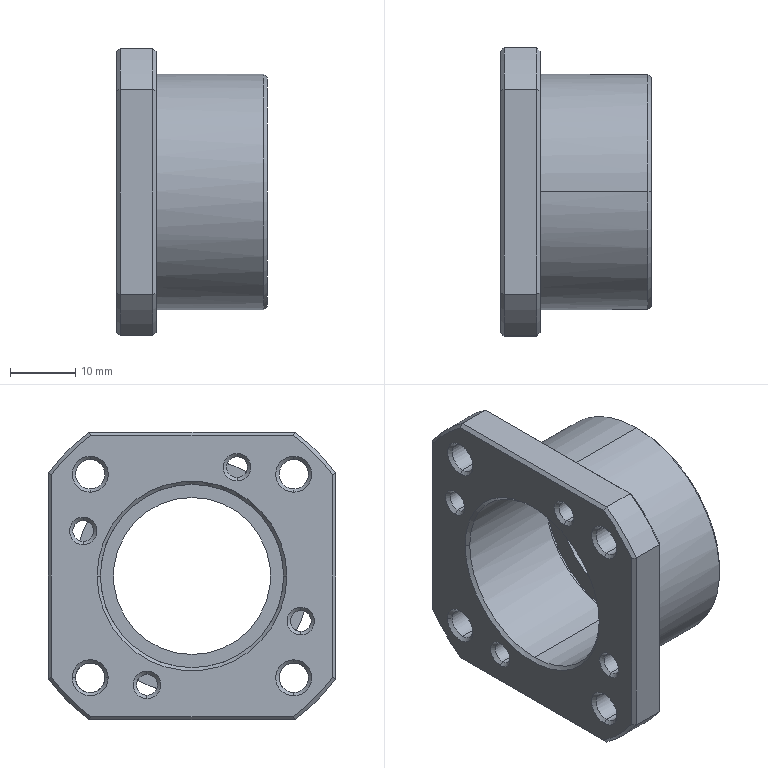Part | STEP file | LFK12-1 | 1 solid | 87 faces | box 23 x 44 x 44 mm | volume 14384 mm3 | cone 38 | cylinder 28 | plane 21 | commonest cylinder face diameters 3.2 x8 4.5 x8 54 x4 24 x2 28 x2 30 x2